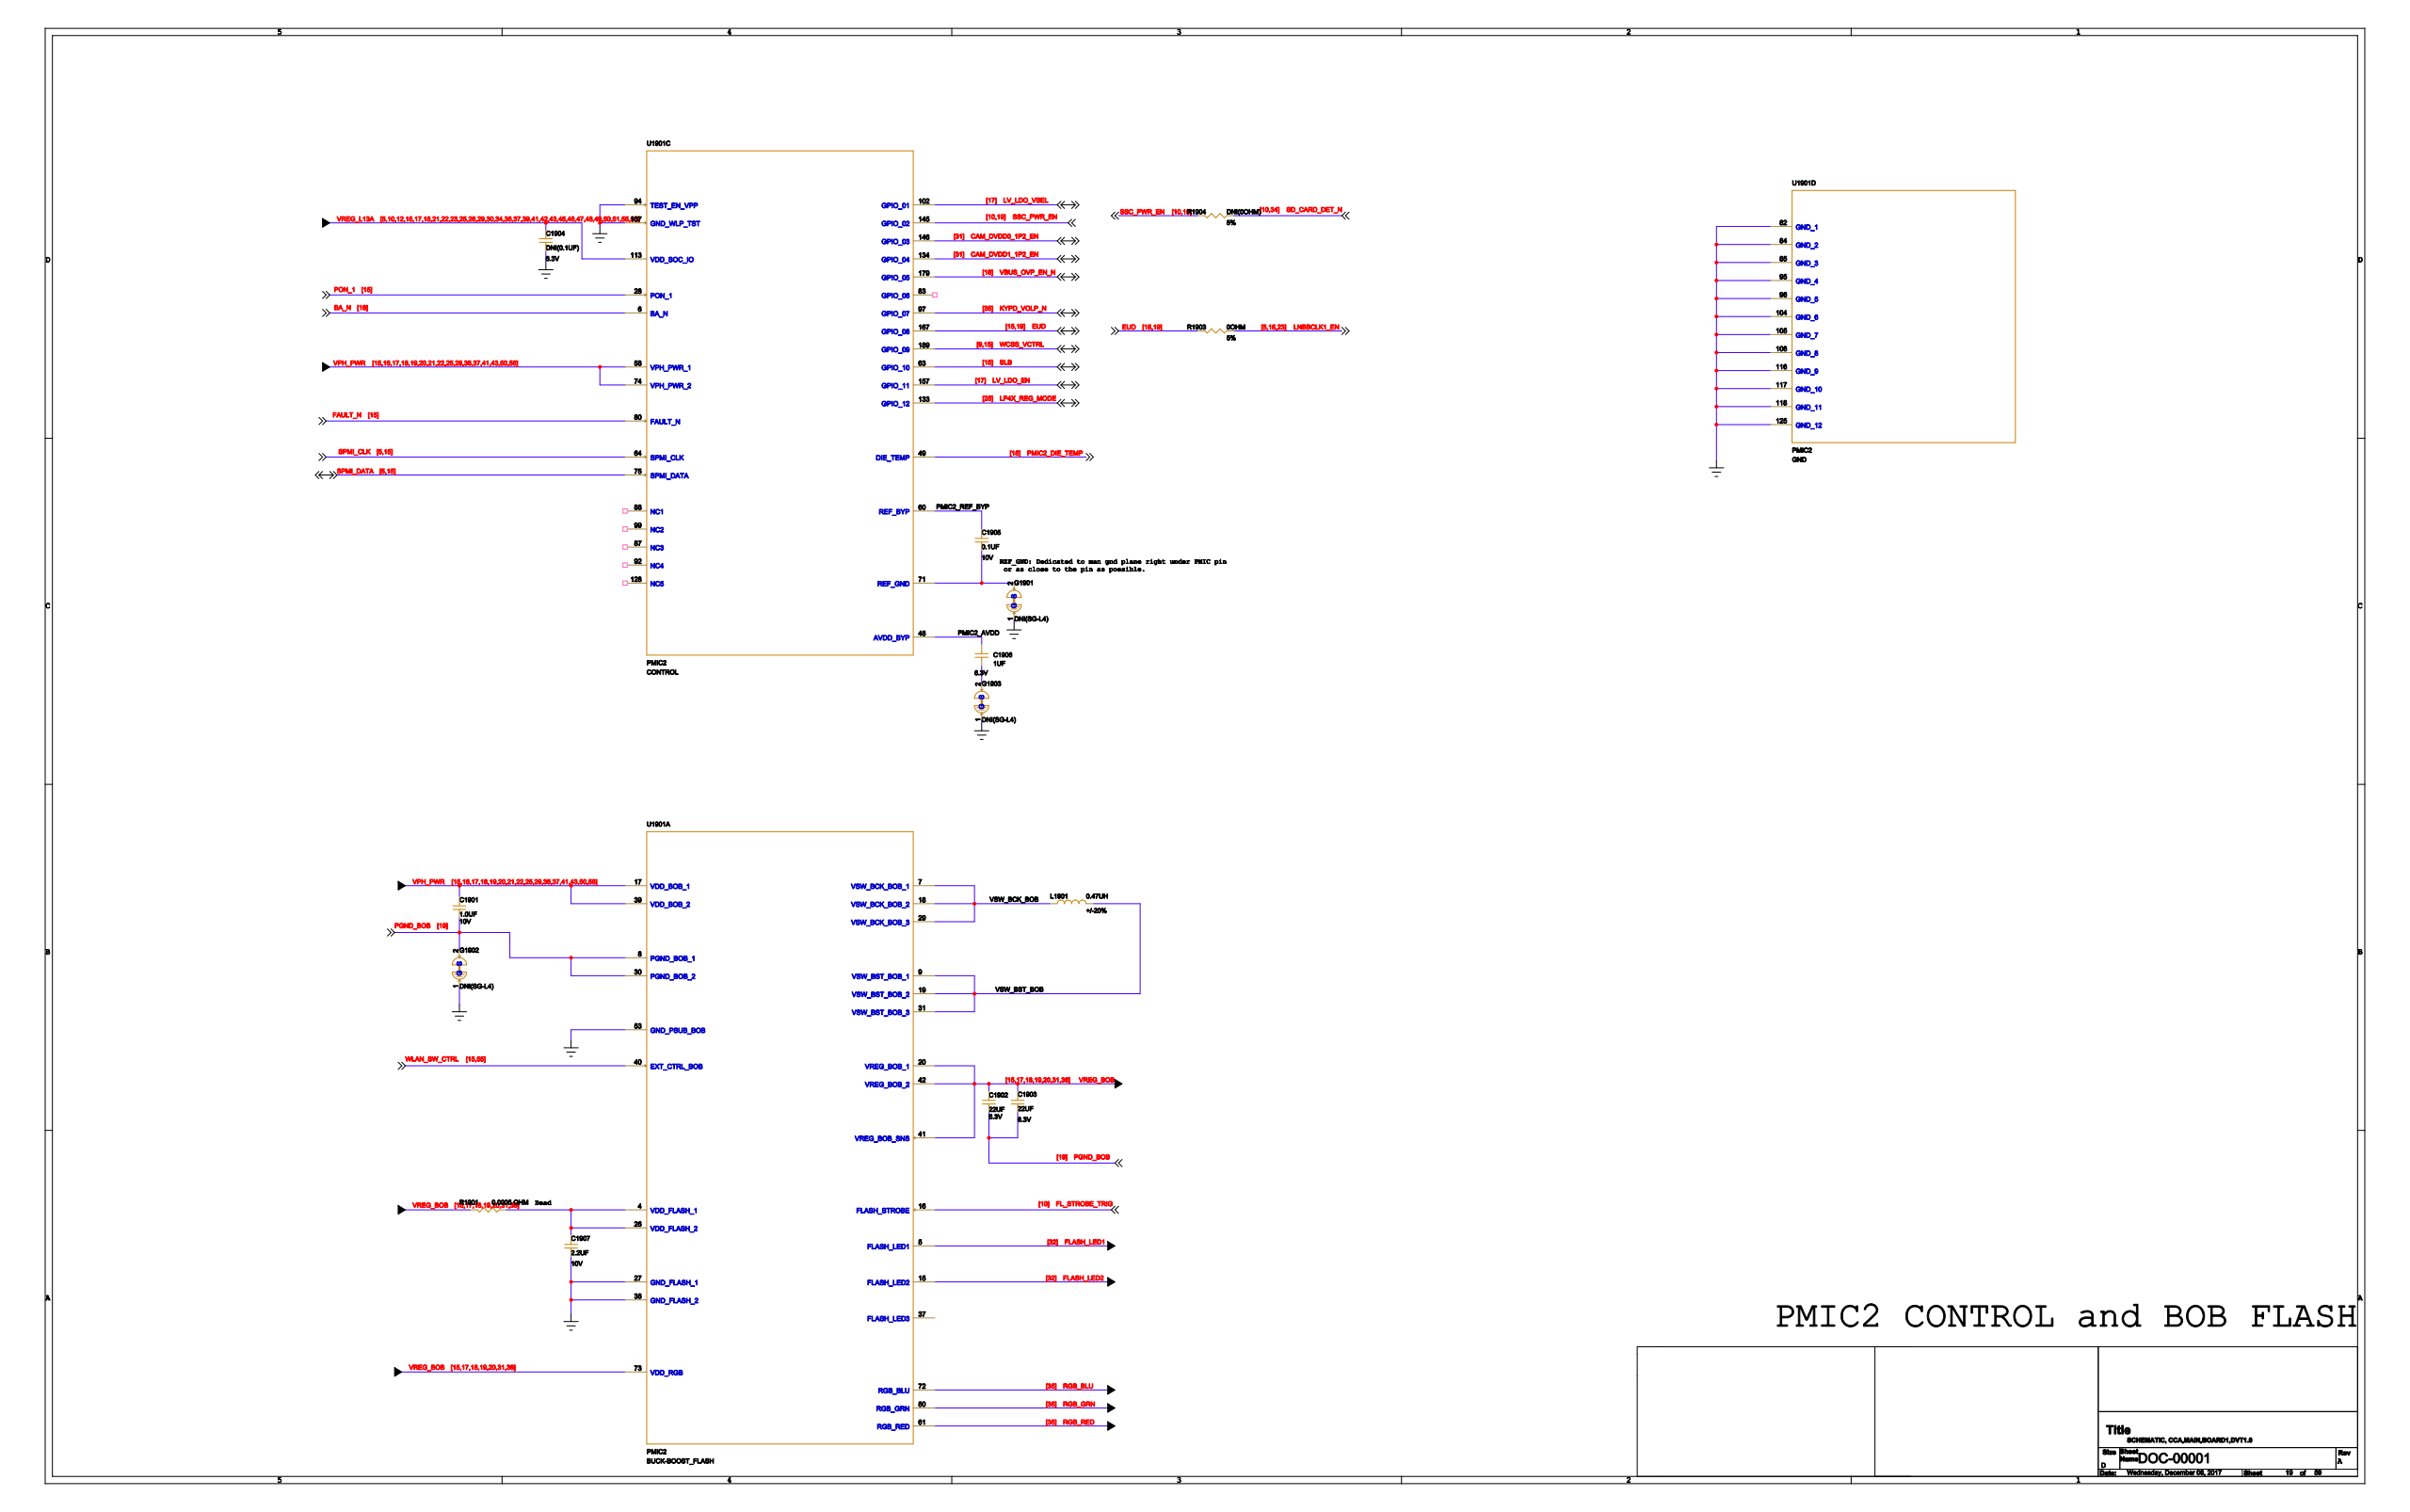Circuit board | KiCad | 1657 parts | 1365 nets | one sheet of the schematic
Parts on this sheet (reference | value | footprint):
C1901
C1902
C1903
C1904
C1905
C1906
C1907
G1901
G1902
G1903
L1901
R1901
R1903
R1904
U1901
Nets of these parts (net: part-pin ...):
GND: C1904-2 C1907-1 G1901-1 G1902-1 G1903-1 U1901-27 U1901-38 U1901-53 U1901-82 U1901-84 U1901-85 U1901-94 U1901-95 U1901-96 U1901-104 U1901-105 U1901-106 U1901-107 U1901-116 U1901-117 U1901-118 U1901-125
VREG_L13A: C1904-1 U1901-113
VPH_PWR: C1901-2 U1901-2 U1901-17 U1901-21 U1901-39 U1901-58 U1901-74
SD_CARD_DET_N: R1904-2
LNBBCLK1_EN: R1903-2
VREG_BOB: C1902-2 C1903-2 R1901-1 U1901-20 U1901-25 U1901-41 U1901-42 U1901-73
N42472694: C1906-1 G1903-2
SPMI_CLK: U1901-64
WLAN_SW_CTRL: U1901-40
LP4X_REG_MODE: U1901-133
PGND_BOB: C1901-1 C1902-1 C1903-1 G1902-2 U1901-8 U1901-30
N39245693: C1905-1 G1901-2 U1901-71
RGB_BLU: U1901-72
RGB_RED: U1901-61
RGB_GRN: U1901-50
VBUS_OVP_EN_N: U1901-179
SPMI_DATA: U1901-75
FL_STROBE_TRIG: U1901-16
WCSS_VCTRL: U1901-189
SSC_PWR_EN: R1904-1 U1901-145
LV_LDO_VSEL: U1901-102
LV_LDO_EN: U1901-157
N24091595: C1907-2 R1901-2 U1901-4 U1901-26
FLASH_LED1: U1901-5
EUD: R1903-1 U1901-167
VSW_BCK_BOB: L1901-1 U1901-7 U1901-18 U1901-29
VSW_BST_BOB: L1901-2 U1901-9 U1901-19 U1901-31
FAULT_N: U1901-80
BA_N: U1901-6
FLASH_LED2: U1901-15
PON_1: U1901-28
FLASH_LED3: U1901-37
PMIC2_AVDD: C1906-2 U1901-48
PMIC2_DIE_TEMP: U1901-49
PMIC2_REF_BYP: C1905-2 U1901-60
SLB: U1901-63
KYPD_VOLP_N: U1901-97